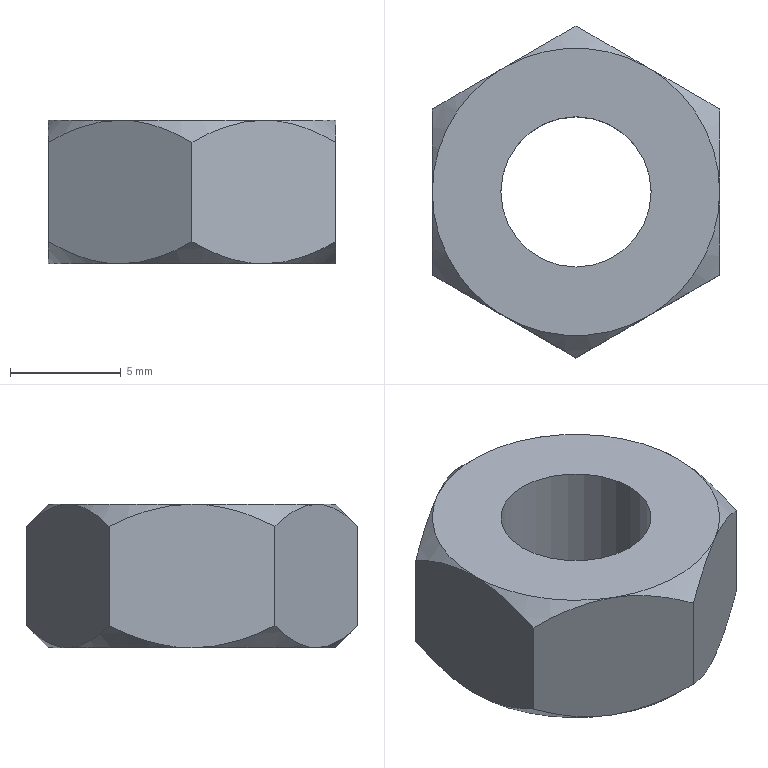Part | NX | 1 solid | 22 faces | box 13 x 15.011 x 6.5 mm | volume 707.016 mm3 | cone 12 | plane 8 | cylinder 2 | commonest cylinder face diameters 6.8 x2
STEP:
#1=CARTESIAN_POINT('',(3.25,-5.629,-3.25));
#2=VERTEX_POINT('',#1);
#3=CARTESIAN_POINT('',(6.5,0.,-3.25));
#4=VERTEX_POINT('',#3);
#5=CARTESIAN_POINT('',(0.,0.,-3.25));
#6=DIRECTION('',(0.,0.,1.));
#7=DIRECTION('',(0.5,-0.866,0.));
#8=AXIS2_PLACEMENT_3D('',#5,#6,#7);
#9=CIRCLE('',#8,6.5);
#10=EDGE_CURVE('',#2,#4,#9,.T.);
#11=ORIENTED_EDGE('',*,*,#10,.F.);
#12=CARTESIAN_POINT('',(-3.25,-5.629,-3.25));
#13=VERTEX_POINT('',#12);
#14=CARTESIAN_POINT('',(0.,0.,-3.25));
#15=DIRECTION('',(0.,0.,1.));
#16=DIRECTION('',(-0.5,-0.866,0.));
#17=AXIS2_PLACEMENT_3D('',#14,#15,#16);
#18=CIRCLE('',#17,6.5);
#19=EDGE_CURVE('',#13,#2,#18,.T.);
#20=ORIENTED_EDGE('',*,*,#19,.F.);
#21=CARTESIAN_POINT('',(-6.5,0.,-3.25));
#22=VERTEX_POINT('',#21);
#23=CARTESIAN_POINT('',(0.,0.,-3.25));
#24=DIRECTION('',(0.,0.,1.));
#25=DIRECTION('',(-1.,0.,0.));
#26=AXIS2_PLACEMENT_3D('',#23,#24,#25);
#27=CIRCLE('',#26,6.5);
#28=EDGE_CURVE('',#22,#13,#27,.T.);
#29=ORIENTED_EDGE('',*,*,#28,.F.);
#30=CARTESIAN_POINT('',(-3.25,5.629,-3.25));
#31=VERTEX_POINT('',#30);
#32=CARTESIAN_POINT('',(0.,0.,-3.25));
#33=DIRECTION('',(0.,0.,1.));
#34=DIRECTION('',(-0.5,0.866,0.));
#35=AXIS2_PLACEMENT_3D('',#32,#33,#34);
#36=CIRCLE('',#35,6.5);
#37=EDGE_CURVE('',#31,#22,#36,.T.);
#38=ORIENTED_EDGE('',*,*,#37,.F.);
#39=CARTESIAN_POINT('',(3.25,5.629,-3.25));
#40=VERTEX_POINT('',#39);
#41=CARTESIAN_POINT('',(0.,0.,-3.25));
#42=DIRECTION('',(0.,0.,1.));
#43=DIRECTION('',(0.5,0.866,0.));
#44=AXIS2_PLACEMENT_3D('',#41,#42,#43);
#45=CIRCLE('',#44,6.5);
#46=EDGE_CURVE('',#40,#31,#45,.T.);
#47=ORIENTED_EDGE('',*,*,#46,.F.);
#48=CARTESIAN_POINT('',(0.,0.,-3.25));
#49=DIRECTION('',(0.,0.,1.));
#50=DIRECTION('',(1.,0.,0.));
#51=AXIS2_PLACEMENT_3D('',#48,#49,#50);
#52=CIRCLE('',#51,6.5);
#53=EDGE_CURVE('',#4,#40,#52,.T.);
#54=ORIENTED_EDGE('',*,*,#53,.F.);
#55=EDGE_LOOP('',(#11,#20,#29,#38,#47,#54));
#56=FACE_BOUND('',#55,.T.);
#57=CARTESIAN_POINT('',(3.4,0.,-3.25));
#58=VERTEX_POINT('',#57);
#59=CARTESIAN_POINT('',(-3.4,0.,-3.25));
#60=VERTEX_POINT('',#59);
#61=CARTESIAN_POINT('',(0.,0.,-3.25));
#62=DIRECTION('',(0.,0.,-1.));
#63=DIRECTION('',(-1.,0.,0.));
#64=AXIS2_PLACEMENT_3D('',#61,#62,#63);
#65=CIRCLE('',#64,3.4);
#66=EDGE_CURVE('',#58,#60,#65,.T.);
#67=ORIENTED_EDGE('',*,*,#66,.F.);
#68=CARTESIAN_POINT('',(0.,0.,-3.25));
#69=DIRECTION('',(0.,0.,-1.));
#70=DIRECTION('',(-1.,0.,0.));
#71=AXIS2_PLACEMENT_3D('',#68,#69,#70);
#72=CIRCLE('',#71,3.4);
#73=EDGE_CURVE('',#60,#58,#72,.T.);
#74=ORIENTED_EDGE('',*,*,#73,.F.);
#75=EDGE_LOOP('',(#67,#74));
#76=FACE_BOUND('',#75,.T.);
#77=CARTESIAN_POINT('',(0.,0.,-3.25));
#78=DIRECTION('',(0.,0.,1.));
#79=DIRECTION('',(1.,0.,0.));
#80=AXIS2_PLACEMENT_3D('',#77,#78,#79);
#81=PLANE('',#80);
#82=ADVANCED_FACE('',(#56,#76),#81,.F.);
#83=CARTESIAN_POINT('',(6.5,-3.753,-2.244));
#84=VERTEX_POINT('',#83);
#85=CARTESIAN_POINT('',(3.25,-5.629,-3.25));
#86=CARTESIAN_POINT('',(3.764,-5.332,-3.25));
#87=CARTESIAN_POINT('',(4.854,-4.703,-3.071));
#88=CARTESIAN_POINT('',(5.912,-4.092,-2.584));
#89=CARTESIAN_POINT('',(6.5,-3.753,-2.244));
#90=B_SPLINE_CURVE_WITH_KNOTS('',3,(#85,#86,#87,#88,#89),.UNSPECIFIED.,.F.,.F.,(4,1,4),(0.,0.5,1.),.UNSPECIFIED.);
#91=EDGE_CURVE('',#2,#84,#90,.T.);
#92=ORIENTED_EDGE('',*,*,#91,.F.);
#93=ORIENTED_EDGE('',*,*,#10,.T.);
#94=CARTESIAN_POINT('',(6.5,-3.753,-2.244));
#95=CARTESIAN_POINT('',(6.5,-2.364,-2.939));
#96=CARTESIAN_POINT('',(6.5,-1.194,-3.25));
#97=CARTESIAN_POINT('',(6.5,0.,-3.25));
#98=B_SPLINE_CURVE_WITH_KNOTS('',3,(#94,#95,#96,#97),.UNSPECIFIED.,.F.,.F.,(4,4),(0.,1.),.UNSPECIFIED.);
#99=EDGE_CURVE('',#84,#4,#98,.T.);
#100=ORIENTED_EDGE('',*,*,#99,.F.);
#101=EDGE_LOOP('',(#92,#93,#100));
#102=FACE_BOUND('',#101,.T.);
#103=CARTESIAN_POINT('',(0.,0.,-2.747));
#104=DIRECTION('',(0.,0.,1.));
#105=DIRECTION('',(1.,0.,0.));
#106=AXIS2_PLACEMENT_3D('',#103,#104,#105);
#107=CONICAL_SURFACE('',#106,7.003,0.7854);
#108=ADVANCED_FACE('',(#102),#107,.T.);
#109=ORIENTED_EDGE('',*,*,#91,.T.);
#110=CARTESIAN_POINT('',(6.5,-3.753,2.244));
#111=VERTEX_POINT('',#110);
#112=CARTESIAN_POINT('',(6.5,-3.753,2.244));
#113=DIRECTION('',(0.,0.,-1.));
#114=VECTOR('',#113,1000.);
#115=LINE('',#112,#114);
#116=EDGE_CURVE('',#111,#84,#115,.T.);
#117=ORIENTED_EDGE('',*,*,#116,.F.);
#118=CARTESIAN_POINT('',(3.25,-5.629,3.25));
#119=VERTEX_POINT('',#118);
#120=CARTESIAN_POINT('',(6.5,-3.753,2.244));
#121=CARTESIAN_POINT('',(6.238,-3.904,2.396));
#122=CARTESIAN_POINT('',(5.711,-4.208,2.667));
#123=CARTESIAN_POINT('',(5.052,-4.589,2.946));
#124=CARTESIAN_POINT('',(4.099,-5.139,3.205));
#125=CARTESIAN_POINT('',(3.536,-5.464,3.25));
#126=CARTESIAN_POINT('',(3.25,-5.629,3.25));
#127=B_SPLINE_CURVE_WITH_KNOTS('',3,(#120,#121,#122,#123,#124,#125,#126),.UNSPECIFIED.,.F.,.F.,(4,1,1,1,4),(0.,0.25,0.5,0.75,1.),.UNSPECIFIED.);
#128=EDGE_CURVE('',#119,#111,#127,.F.);
#129=ORIENTED_EDGE('',*,*,#128,.F.);
#130=CARTESIAN_POINT('',(0.,-7.506,2.244));
#131=VERTEX_POINT('',#130);
#132=CARTESIAN_POINT('',(3.25,-5.629,3.25));
#133=CARTESIAN_POINT('',(2.736,-5.926,3.25));
#134=CARTESIAN_POINT('',(1.646,-6.555,3.071));
#135=CARTESIAN_POINT('',(0.5876,-7.166,2.584));
#136=CARTESIAN_POINT('',(0.,-7.506,2.244));
#137=B_SPLINE_CURVE_WITH_KNOTS('',3,(#132,#133,#134,#135,#136),.UNSPECIFIED.,.F.,.F.,(4,1,4),(0.,0.5,1.),.UNSPECIFIED.);
#138=EDGE_CURVE('',#119,#131,#137,.T.);
#139=ORIENTED_EDGE('',*,*,#138,.T.);
#140=CARTESIAN_POINT('',(0.,-7.506,-2.244));
#141=VERTEX_POINT('',#140);
#142=CARTESIAN_POINT('',(0.,-7.506,2.244));
#143=DIRECTION('',(0.,0.,-1.));
#144=VECTOR('',#143,1000.);
#145=LINE('',#142,#144);
#146=EDGE_CURVE('',#131,#141,#145,.T.);
#147=ORIENTED_EDGE('',*,*,#146,.T.);
#148=CARTESIAN_POINT('',(0.,-7.506,-2.244));
#149=CARTESIAN_POINT('',(0.1225,-7.435,-2.315));
#150=CARTESIAN_POINT('',(0.3631,-7.296,-2.448));
#151=CARTESIAN_POINT('',(0.7094,-7.096,-2.622));
#152=CARTESIAN_POINT('',(1.045,-6.902,-2.772));
#153=CARTESIAN_POINT('',(1.372,-6.714,-2.901));
#154=CARTESIAN_POINT('',(1.692,-6.529,-3.009));
#155=CARTESIAN_POINT('',(2.008,-6.346,-3.097));
#156=CARTESIAN_POINT('',(2.321,-6.165,-3.165));
#157=CARTESIAN_POINT('',(2.632,-5.986,-3.214));
#158=CARTESIAN_POINT('',(2.941,-5.807,-3.243));
#159=CARTESIAN_POINT('',(3.147,-5.689,-3.25));
#160=CARTESIAN_POINT('',(3.25,-5.629,-3.25));
#161=B_SPLINE_CURVE_WITH_KNOTS('',3,(#148,#149,#150,#151,#152,#153,#154,#155,#156,#157,#158,#159,#160),.UNSPECIFIED.,.F.,.F.,(4,1,1,1,1,1,1,1,1,1,4),(0.,0.1,0.2,0.3,0.4,0.5,0.6,0.7,0.8,0.9,1.),.UNSPECIFIED.);
#162=EDGE_CURVE('',#141,#2,#161,.T.);
#163=ORIENTED_EDGE('',*,*,#162,.T.);
#164=EDGE_LOOP('',(#109,#117,#129,#139,#147,#163));
#165=FACE_BOUND('',#164,.T.);
#166=CARTESIAN_POINT('',(0.,-7.506,-3.25));
#167=DIRECTION('',(0.5,-0.866,0.));
#168=DIRECTION('',(0.,0.,-1.));
#169=AXIS2_PLACEMENT_3D('',#166,#167,#168);
#170=PLANE('',#169);
#171=ADVANCED_FACE('',(#165),#170,.T.);
#172=CARTESIAN_POINT('',(-3.25,-5.629,-3.25));
#173=CARTESIAN_POINT('',(-2.736,-5.926,-3.25));
#174=CARTESIAN_POINT('',(-1.646,-6.555,-3.071));
#175=CARTESIAN_POINT('',(-0.5876,-7.166,-2.584));
#176=CARTESIAN_POINT('',(0.,-7.506,-2.244));
#177=B_SPLINE_CURVE_WITH_KNOTS('',3,(#172,#173,#174,#175,#176),.UNSPECIFIED.,.F.,.F.,(4,1,4),(0.,0.5,1.),.UNSPECIFIED.);
#178=EDGE_CURVE('',#13,#141,#177,.T.);
#179=ORIENTED_EDGE('',*,*,#178,.F.);
#180=ORIENTED_EDGE('',*,*,#19,.T.);
#181=ORIENTED_EDGE('',*,*,#162,.F.);
#182=EDGE_LOOP('',(#179,#180,#181));
#183=FACE_BOUND('',#182,.T.);
#184=CARTESIAN_POINT('',(0.,0.,-2.747));
#185=DIRECTION('',(0.,0.,1.));
#186=DIRECTION('',(1.,0.,0.));
#187=AXIS2_PLACEMENT_3D('',#184,#185,#186);
#188=CONICAL_SURFACE('',#187,7.003,0.7854);
#189=ADVANCED_FACE('',(#183),#188,.T.);
#190=ORIENTED_EDGE('',*,*,#178,.T.);
#191=ORIENTED_EDGE('',*,*,#146,.F.);
#192=CARTESIAN_POINT('',(-3.25,-5.629,3.25));
#193=VERTEX_POINT('',#192);
#194=CARTESIAN_POINT('',(0.,-7.506,2.244));
#195=CARTESIAN_POINT('',(-0.2618,-7.354,2.396));
#196=CARTESIAN_POINT('',(-0.7889,-7.05,2.667));
#197=CARTESIAN_POINT('',(-1.448,-6.669,2.946));
#198=CARTESIAN_POINT('',(-2.401,-6.119,3.205));
#199=CARTESIAN_POINT('',(-2.964,-5.794,3.25));
#200=CARTESIAN_POINT('',(-3.25,-5.629,3.25));
#201=B_SPLINE_CURVE_WITH_KNOTS('',3,(#194,#195,#196,#197,#198,#199,#200),.UNSPECIFIED.,.F.,.F.,(4,1,1,1,4),(0.,0.25,0.5,0.75,1.),.UNSPECIFIED.);
#202=EDGE_CURVE('',#193,#131,#201,.F.);
#203=ORIENTED_EDGE('',*,*,#202,.F.);
#204=CARTESIAN_POINT('',(-6.5,-3.753,2.244));
#205=VERTEX_POINT('',#204);
#206=CARTESIAN_POINT('',(-3.25,-5.629,3.25));
#207=CARTESIAN_POINT('',(-3.764,-5.332,3.25));
#208=CARTESIAN_POINT('',(-4.854,-4.703,3.071));
#209=CARTESIAN_POINT('',(-5.912,-4.092,2.584));
#210=CARTESIAN_POINT('',(-6.5,-3.753,2.244));
#211=B_SPLINE_CURVE_WITH_KNOTS('',3,(#206,#207,#208,#209,#210),.UNSPECIFIED.,.F.,.F.,(4,1,4),(0.,0.5,1.),.UNSPECIFIED.);
#212=EDGE_CURVE('',#193,#205,#211,.T.);
#213=ORIENTED_EDGE('',*,*,#212,.T.);
#214=CARTESIAN_POINT('',(-6.5,-3.753,-2.244));
#215=VERTEX_POINT('',#214);
#216=CARTESIAN_POINT('',(-6.5,-3.753,2.244));
#217=DIRECTION('',(0.,0.,-1.));
#218=VECTOR('',#217,1000.);
#219=LINE('',#216,#218);
#220=EDGE_CURVE('',#205,#215,#219,.T.);
#221=ORIENTED_EDGE('',*,*,#220,.T.);
#222=CARTESIAN_POINT('',(-6.5,-3.753,-2.244));
#223=CARTESIAN_POINT('',(-6.378,-3.823,-2.315));
#224=CARTESIAN_POINT('',(-6.137,-3.962,-2.448));
#225=CARTESIAN_POINT('',(-5.791,-4.162,-2.622));
#226=CARTESIAN_POINT('',(-5.455,-4.356,-2.772));
#227=CARTESIAN_POINT('',(-5.128,-4.545,-2.901));
#228=CARTESIAN_POINT('',(-4.808,-4.73,-3.009));
#229=CARTESIAN_POINT('',(-4.492,-4.912,-3.097));
#230=CARTESIAN_POINT('',(-4.179,-5.093,-3.165));
#231=CARTESIAN_POINT('',(-3.868,-5.272,-3.214));
#232=CARTESIAN_POINT('',(-3.559,-5.451,-3.243));
#233=CARTESIAN_POINT('',(-3.353,-5.57,-3.25));
#234=CARTESIAN_POINT('',(-3.25,-5.629,-3.25));
#235=B_SPLINE_CURVE_WITH_KNOTS('',3,(#222,#223,#224,#225,#226,#227,#228,#229,#230,#231,#232,#233,#234),.UNSPECIFIED.,.F.,.F.,(4,1,1,1,1,1,1,1,1,1,4),(0.,0.1,0.2,0.3,0.4,0.5,0.6,0.7,0.8,0.9,1.),.UNSPECIFIED.);
#236=EDGE_CURVE('',#215,#13,#235,.T.);
#237=ORIENTED_EDGE('',*,*,#236,.T.);
#238=EDGE_LOOP('',(#190,#191,#203,#213,#221,#237));
#239=FACE_BOUND('',#238,.T.);
#240=CARTESIAN_POINT('',(-6.5,-3.753,-3.25));
#241=DIRECTION('',(-0.5,-0.866,0.));
#242=DIRECTION('',(-0.866,0.5,0.));
#243=AXIS2_PLACEMENT_3D('',#240,#241,#242);
#244=PLANE('',#243);
#245=ADVANCED_FACE('',(#239),#244,.T.);
#246=CARTESIAN_POINT('',(-6.5,0.,-3.25));
#247=CARTESIAN_POINT('',(-6.5,-0.5936,-3.25));
#248=CARTESIAN_POINT('',(-6.5,-1.851,-3.071));
#249=CARTESIAN_POINT('',(-6.5,-3.074,-2.584));
#250=CARTESIAN_POINT('',(-6.5,-3.753,-2.244));
#251=B_SPLINE_CURVE_WITH_KNOTS('',3,(#246,#247,#248,#249,#250),.UNSPECIFIED.,.F.,.F.,(4,1,4),(0.,0.5,1.),.UNSPECIFIED.);
#252=EDGE_CURVE('',#22,#215,#251,.T.);
#253=ORIENTED_EDGE('',*,*,#252,.F.);
#254=ORIENTED_EDGE('',*,*,#28,.T.);
#255=ORIENTED_EDGE('',*,*,#236,.F.);
#256=EDGE_LOOP('',(#253,#254,#255));
#257=FACE_BOUND('',#256,.T.);
#258=CARTESIAN_POINT('',(0.,0.,-2.747));
#259=DIRECTION('',(0.,0.,1.));
#260=DIRECTION('',(1.,0.,0.));
#261=AXIS2_PLACEMENT_3D('',#258,#259,#260);
#262=CONICAL_SURFACE('',#261,7.003,0.7854);
#263=ADVANCED_FACE('',(#257),#262,.T.);
#264=ORIENTED_EDGE('',*,*,#252,.T.);
#265=ORIENTED_EDGE('',*,*,#220,.F.);
#266=CARTESIAN_POINT('',(-6.5,0.,3.25));
#267=VERTEX_POINT('',#266);
#268=CARTESIAN_POINT('',(-6.5,-3.753,2.244));
#269=CARTESIAN_POINT('',(-6.5,-3.447,2.397));
#270=CARTESIAN_POINT('',(-6.5,-2.834,2.671));
#271=CARTESIAN_POINT('',(-6.5,-2.057,2.953));
#272=CARTESIAN_POINT('',(-6.5,-0.9732,3.205));
#273=CARTESIAN_POINT('',(-6.5,-0.3273,3.25));
#274=CARTESIAN_POINT('',(-6.5,0.,3.25));
#275=B_SPLINE_CURVE_WITH_KNOTS('',3,(#268,#269,#270,#271,#272,#273,#274),.UNSPECIFIED.,.F.,.F.,(4,1,1,1,4),(0.,0.25,0.5,0.75,1.),.UNSPECIFIED.);
#276=EDGE_CURVE('',#267,#205,#275,.F.);
#277=ORIENTED_EDGE('',*,*,#276,.F.);
#278=CARTESIAN_POINT('',(-6.5,3.753,2.244));
#279=VERTEX_POINT('',#278);
#280=CARTESIAN_POINT('',(-6.5,0.,3.25));
#281=CARTESIAN_POINT('',(-6.5,0.5936,3.25));
#282=CARTESIAN_POINT('',(-6.5,1.851,3.071));
#283=CARTESIAN_POINT('',(-6.5,3.074,2.584));
#284=CARTESIAN_POINT('',(-6.5,3.753,2.244));
#285=B_SPLINE_CURVE_WITH_KNOTS('',3,(#280,#281,#282,#283,#284),.UNSPECIFIED.,.F.,.F.,(4,1,4),(0.,0.5,1.),.UNSPECIFIED.);
#286=EDGE_CURVE('',#267,#279,#285,.T.);
#287=ORIENTED_EDGE('',*,*,#286,.T.);
#288=CARTESIAN_POINT('',(-6.5,3.753,-2.244));
#289=VERTEX_POINT('',#288);
#290=CARTESIAN_POINT('',(-6.5,3.753,2.244));
#291=DIRECTION('',(0.,0.,-1.));
#292=VECTOR('',#291,1000.);
#293=LINE('',#290,#292);
#294=EDGE_CURVE('',#279,#289,#293,.T.);
#295=ORIENTED_EDGE('',*,*,#294,.T.);
#296=CARTESIAN_POINT('',(-6.5,3.753,-2.244));
#297=CARTESIAN_POINT('',(-6.5,2.364,-2.939));
#298=CARTESIAN_POINT('',(-6.5,1.194,-3.25));
#299=CARTESIAN_POINT('',(-6.5,0.,-3.25));
#300=B_SPLINE_CURVE_WITH_KNOTS('',3,(#296,#297,#298,#299),.UNSPECIFIED.,.F.,.F.,(4,4),(0.,1.),.UNSPECIFIED.);
#301=EDGE_CURVE('',#289,#22,#300,.T.);
#302=ORIENTED_EDGE('',*,*,#301,.T.);
#303=EDGE_LOOP('',(#264,#265,#277,#287,#295,#302));
#304=FACE_BOUND('',#303,.T.);
#305=CARTESIAN_POINT('',(-6.5,3.753,-3.25));
#306=DIRECTION('',(-1.,0.,0.));
#307=DIRECTION('',(0.,0.,1.));
#308=AXIS2_PLACEMENT_3D('',#305,#306,#307);
#309=PLANE('',#308);
#310=ADVANCED_FACE('',(#304),#309,.T.);
#311=CARTESIAN_POINT('',(-3.25,5.629,-3.25));
#312=CARTESIAN_POINT('',(-3.764,5.332,-3.25));
#313=CARTESIAN_POINT('',(-4.854,4.703,-3.071));
#314=CARTESIAN_POINT('',(-5.912,4.092,-2.584));
#315=CARTESIAN_POINT('',(-6.5,3.753,-2.244));
#316=B_SPLINE_CURVE_WITH_KNOTS('',3,(#311,#312,#313,#314,#315),.UNSPECIFIED.,.F.,.F.,(4,1,4),(0.,0.5,1.),.UNSPECIFIED.);
#317=EDGE_CURVE('',#31,#289,#316,.T.);
#318=ORIENTED_EDGE('',*,*,#317,.F.);
#319=ORIENTED_EDGE('',*,*,#37,.T.);
#320=ORIENTED_EDGE('',*,*,#301,.F.);
#321=EDGE_LOOP('',(#318,#319,#320));
#322=FACE_BOUND('',#321,.T.);
#323=CARTESIAN_POINT('',(0.,0.,-2.747));
#324=DIRECTION('',(0.,0.,1.));
#325=DIRECTION('',(1.,0.,0.));
#326=AXIS2_PLACEMENT_3D('',#323,#324,#325);
#327=CONICAL_SURFACE('',#326,7.003,0.7854);
#328=ADVANCED_FACE('',(#322),#327,.T.);
#329=ORIENTED_EDGE('',*,*,#317,.T.);
#330=ORIENTED_EDGE('',*,*,#294,.F.);
#331=CARTESIAN_POINT('',(-3.25,5.629,3.25));
#332=VERTEX_POINT('',#331);
#333=CARTESIAN_POINT('',(-6.5,3.753,2.244));
#334=CARTESIAN_POINT('',(-6.238,3.904,2.396));
#335=CARTESIAN_POINT('',(-5.711,4.208,2.667));
#336=CARTESIAN_POINT('',(-5.052,4.589,2.946));
#337=CARTESIAN_POINT('',(-4.099,5.139,3.205));
#338=CARTESIAN_POINT('',(-3.536,5.464,3.25));
#339=CARTESIAN_POINT('',(-3.25,5.629,3.25));
#340=B_SPLINE_CURVE_WITH_KNOTS('',3,(#333,#334,#335,#336,#337,#338,#339),.UNSPECIFIED.,.F.,.F.,(4,1,1,1,4),(0.,0.25,0.5,0.75,1.),.UNSPECIFIED.);
#341=EDGE_CURVE('',#332,#279,#340,.F.);
#342=ORIENTED_EDGE('',*,*,#341,.F.);
#343=CARTESIAN_POINT('',(0.,7.506,2.244));
#344=VERTEX_POINT('',#343);
#345=CARTESIAN_POINT('',(-3.25,5.629,3.25));
#346=CARTESIAN_POINT('',(-2.736,5.926,3.25));
#347=CARTESIAN_POINT('',(-1.646,6.555,3.071));
#348=CARTESIAN_POINT('',(-0.5876,7.166,2.584));
#349=CARTESIAN_POINT('',(0.,7.506,2.244));
#350=B_SPLINE_CURVE_WITH_KNOTS('',3,(#345,#346,#347,#348,#349),.UNSPECIFIED.,.F.,.F.,(4,1,4),(0.,0.5,1.),.UNSPECIFIED.);
#351=EDGE_CURVE('',#332,#344,#350,.T.);
#352=ORIENTED_EDGE('',*,*,#351,.T.);
#353=CARTESIAN_POINT('',(0.,7.506,-2.244));
#354=VERTEX_POINT('',#353);
#355=CARTESIAN_POINT('',(0.,7.506,2.244));
#356=DIRECTION('',(0.,0.,-1.));
#357=VECTOR('',#356,1000.);
#358=LINE('',#355,#357);
#359=EDGE_CURVE('',#344,#354,#358,.T.);
#360=ORIENTED_EDGE('',*,*,#359,.T.);
#361=CARTESIAN_POINT('',(0.,7.506,-2.244));
#362=CARTESIAN_POINT('',(-0.1225,7.435,-2.315));
#363=CARTESIAN_POINT('',(-0.3631,7.296,-2.448));
#364=CARTESIAN_POINT('',(-0.7094,7.096,-2.622));
#365=CARTESIAN_POINT('',(-1.045,6.902,-2.772));
#366=CARTESIAN_POINT('',(-1.372,6.714,-2.901));
#367=CARTESIAN_POINT('',(-1.692,6.529,-3.009));
#368=CARTESIAN_POINT('',(-2.008,6.346,-3.097));
#369=CARTESIAN_POINT('',(-2.321,6.165,-3.165));
#370=CARTESIAN_POINT('',(-2.632,5.986,-3.214));
#371=CARTESIAN_POINT('',(-2.941,5.807,-3.243));
#372=CARTESIAN_POINT('',(-3.147,5.689,-3.25));
#373=CARTESIAN_POINT('',(-3.25,5.629,-3.25));
#374=B_SPLINE_CURVE_WITH_KNOTS('',3,(#361,#362,#363,#364,#365,#366,#367,#368,#369,#370,#371,#372,#373),.UNSPECIFIED.,.F.,.F.,(4,1,1,1,1,1,1,1,1,1,4),(0.,0.1,0.2,0.3,0.4,0.5,0.6,0.7,0.8,0.9,1.),.UNSPECIFIED.);
#375=EDGE_CURVE('',#354,#31,#374,.T.);
#376=ORIENTED_EDGE('',*,*,#375,.T.);
#377=EDGE_LOOP('',(#329,#330,#342,#352,#360,#376));
#378=FACE_BOUND('',#377,.T.);
#379=CARTESIAN_POINT('',(0.,7.506,-3.25));
#380=DIRECTION('',(-0.5,0.866,0.));
#381=DIRECTION('',(0.,0.,1.));
#382=AXIS2_PLACEMENT_3D('',#379,#380,#381);
#383=PLANE('',#382);
#384=ADVANCED_FACE('',(#378),#383,.T.);
#385=CARTESIAN_POINT('',(3.25,5.629,-3.25));
#386=CARTESIAN_POINT('',(2.736,5.926,-3.25));
#387=CARTESIAN_POINT('',(1.646,6.555,-3.071));
#388=CARTESIAN_POINT('',(0.5876,7.166,-2.584));
#389=CARTESIAN_POINT('',(0.,7.506,-2.244));
#390=B_SPLINE_CURVE_WITH_KNOTS('',3,(#385,#386,#387,#388,#389),.UNSPECIFIED.,.F.,.F.,(4,1,4),(0.,0.5,1.),.UNSPECIFIED.);
#391=EDGE_CURVE('',#40,#354,#390,.T.);
#392=ORIENTED_EDGE('',*,*,#391,.F.);
#393=ORIENTED_EDGE('',*,*,#46,.T.);
#394=ORIENTED_EDGE('',*,*,#375,.F.);
#395=EDGE_LOOP('',(#392,#393,#394));
#396=FACE_BOUND('',#395,.T.);
#397=CARTESIAN_POINT('',(0.,0.,-2.747));
#398=DIRECTION('',(0.,0.,1.));
#399=DIRECTION('',(1.,0.,0.));
#400=AXIS2_PLACEMENT_3D('',#397,#398,#399);
#401=CONICAL_SURFACE('',#400,7.003,0.7854);
#402=ADVANCED_FACE('',(#396),#401,.T.);
#403=ORIENTED_EDGE('',*,*,#391,.T.);
#404=ORIENTED_EDGE('',*,*,#359,.F.);
#405=CARTESIAN_POINT('',(3.25,5.629,3.25));
#406=VERTEX_POINT('',#405);
#407=CARTESIAN_POINT('',(0.,7.506,2.244));
#408=CARTESIAN_POINT('',(0.2618,7.354,2.396));
#409=CARTESIAN_POINT('',(0.7889,7.05,2.667));
#410=CARTESIAN_POINT('',(1.448,6.669,2.946));
#411=CARTESIAN_POINT('',(2.401,6.119,3.205));
#412=CARTESIAN_POINT('',(2.964,5.794,3.25));
#413=CARTESIAN_POINT('',(3.25,5.629,3.25));
#414=B_SPLINE_CURVE_WITH_KNOTS('',3,(#407,#408,#409,#410,#411,#412,#413),.UNSPECIFIED.,.F.,.F.,(4,1,1,1,4),(0.,0.25,0.5,0.75,1.),.UNSPECIFIED.);
#415=EDGE_CURVE('',#406,#344,#414,.F.);
#416=ORIENTED_EDGE('',*,*,#415,.F.);
#417=CARTESIAN_POINT('',(6.5,3.753,2.244));
#418=VERTEX_POINT('',#417);
#419=CARTESIAN_POINT('',(3.25,5.629,3.25));
#420=CARTESIAN_POINT('',(3.764,5.332,3.25));
#421=CARTESIAN_POINT('',(4.854,4.703,3.071));
#422=CARTESIAN_POINT('',(5.912,4.092,2.584));
#423=CARTESIAN_POINT('',(6.5,3.753,2.244));
#424=B_SPLINE_CURVE_WITH_KNOTS('',3,(#419,#420,#421,#422,#423),.UNSPECIFIED.,.F.,.F.,(4,1,4),(0.,0.5,1.),.UNSPECIFIED.);
#425=EDGE_CURVE('',#406,#418,#424,.T.);
#426=ORIENTED_EDGE('',*,*,#425,.T.);
#427=CARTESIAN_POINT('',(6.5,3.753,-2.244));
#428=VERTEX_POINT('',#427);
#429=CARTESIAN_POINT('',(6.5,3.753,2.244));
#430=DIRECTION('',(0.,0.,-1.));
#431=VECTOR('',#430,1000.);
#432=LINE('',#429,#431);
#433=EDGE_CURVE('',#418,#428,#432,.T.);
#434=ORIENTED_EDGE('',*,*,#433,.T.);
#435=CARTESIAN_POINT('',(6.5,3.753,-2.244));
#436=CARTESIAN_POINT('',(6.378,3.823,-2.315));
#437=CARTESIAN_POINT('',(6.137,3.962,-2.448));
#438=CARTESIAN_POINT('',(5.791,4.162,-2.622));
#439=CARTESIAN_POINT('',(5.455,4.356,-2.772));
#440=CARTESIAN_POINT('',(5.128,4.545,-2.901));
#441=CARTESIAN_POINT('',(4.808,4.73,-3.009));
#442=CARTESIAN_POINT('',(4.492,4.912,-3.097));
#443=CARTESIAN_POINT('',(4.179,5.093,-3.165));
#444=CARTESIAN_POINT('',(3.868,5.272,-3.214));
#445=CARTESIAN_POINT('',(3.559,5.451,-3.243));
#446=CARTESIAN_POINT('',(3.353,5.57,-3.25));
#447=CARTESIAN_POINT('',(3.25,5.629,-3.25));
#448=B_SPLINE_CURVE_WITH_KNOTS('',3,(#435,#436,#437,#438,#439,#440,#441,#442,#443,#444,#445,#446,#447),.UNSPECIFIED.,.F.,.F.,(4,1,1,1,1,1,1,1,1,1,4),(0.,0.1,0.2,0.3,0.4,0.5,0.6,0.7,0.8,0.9,1.),.UNSPECIFIED.);
#449=EDGE_CURVE('',#428,#40,#448,.T.);
#450=ORIENTED_EDGE('',*,*,#449,.T.);
#451=EDGE_LOOP('',(#403,#404,#416,#426,#434,#450));
#452=FACE_BOUND('',#451,.T.);
#453=CARTESIAN_POINT('',(6.5,3.753,-3.25));
#454=DIRECTION('',(0.5,0.866,0.));
#455=DIRECTION('',(0.,0.,-1.));
#456=AXIS2_PLACEMENT_3D('',#453,#454,#455);
#457=PLANE('',#456);
#458=ADVANCED_FACE('',(#452),#457,.T.);
#459=CARTESIAN_POINT('',(6.5,0.,-3.25));
#460=CARTESIAN_POINT('',(6.5,0.5936,-3.25));
#461=CARTESIAN_POINT('',(6.5,1.851,-3.071));
#462=CARTESIAN_POINT('',(6.5,3.074,-2.584));
#463=CARTESIAN_POINT('',(6.5,3.753,-2.244));
#464=B_SPLINE_CURVE_WITH_KNOTS('',3,(#459,#460,#461,#462,#463),.UNSPECIFIED.,.F.,.F.,(4,1,4),(0.,0.5,1.),.UNSPECIFIED.);
#465=EDGE_CURVE('',#4,#428,#464,.T.);
#466=ORIENTED_EDGE('',*,*,#465,.F.);
#467=ORIENTED_EDGE('',*,*,#53,.T.);
#468=ORIENTED_EDGE('',*,*,#449,.F.);
#469=EDGE_LOOP('',(#466,#467,#468));
#470=FACE_BOUND('',#469,.T.);
#471=CARTESIAN_POINT('',(0.,0.,-2.747));
#472=DIRECTION('',(0.,0.,1.));
#473=DIRECTION('',(1.,0.,0.));
#474=AXIS2_PLACEMENT_3D('',#471,#472,#473);
#475=CONICAL_SURFACE('',#474,7.003,0.7854);
#476=ADVANCED_FACE('',(#470),#475,.T.);
#477=ORIENTED_EDGE('',*,*,#99,.T.);
#478=ORIENTED_EDGE('',*,*,#465,.T.);
#479=ORIENTED_EDGE('',*,*,#433,.F.);
#480=CARTESIAN_POINT('',(6.5,0.,3.25));
#481=VERTEX_POINT('',#480);
#482=CARTESIAN_POINT('',(6.5,3.753,2.244));
#483=CARTESIAN_POINT('',(6.5,3.447,2.397));
#484=CARTESIAN_POINT('',(6.5,2.834,2.671));
#485=CARTESIAN_POINT('',(6.5,2.057,2.953));
#486=CARTESIAN_POINT('',(6.5,0.9732,3.205));
#487=CARTESIAN_POINT('',(6.5,0.3273,3.25));
#488=CARTESIAN_POINT('',(6.5,0.,3.25));
#489=B_SPLINE_CURVE_WITH_KNOTS('',3,(#482,#483,#484,#485,#486,#487,#488),.UNSPECIFIED.,.F.,.F.,(4,1,1,1,4),(0.,0.25,0.5,0.75,1.),.UNSPECIFIED.);
#490=EDGE_CURVE('',#481,#418,#489,.F.);
#491=ORIENTED_EDGE('',*,*,#490,.F.);
#492=CARTESIAN_POINT('',(6.5,0.,3.25));
#493=CARTESIAN_POINT('',(6.5,-0.5936,3.25));
#494=CARTESIAN_POINT('',(6.5,-1.851,3.071));
#495=CARTESIAN_POINT('',(6.5,-3.074,2.584));
#496=CARTESIAN_POINT('',(6.5,-3.753,2.244));
#497=B_SPLINE_CURVE_WITH_KNOTS('',3,(#492,#493,#494,#495,#496),.UNSPECIFIED.,.F.,.F.,(4,1,4),(0.,0.5,1.),.UNSPECIFIED.);
#498=EDGE_CURVE('',#481,#111,#497,.T.);
#499=ORIENTED_EDGE('',*,*,#498,.T.);
#500=ORIENTED_EDGE('',*,*,#116,.T.);
#501=EDGE_LOOP('',(#477,#478,#479,#491,#499,#500));
#502=FACE_BOUND('',#501,.T.);
#503=CARTESIAN_POINT('',(6.5,-3.753,-3.25));
#504=DIRECTION('',(1.,0.,0.));
#505=DIRECTION('',(0.,1.,0.));
#506=AXIS2_PLACEMENT_3D('',#503,#504,#505);
#507=PLANE('',#506);
#508=ADVANCED_FACE('',(#502),#507,.T.);
#509=ORIENTED_EDGE('',*,*,#498,.F.);
#510=CARTESIAN_POINT('',(0.,0.,3.25));
#511=DIRECTION('',(0.,0.,-1.));
#512=DIRECTION('',(1.,0.,0.));
#513=AXIS2_PLACEMENT_3D('',#510,#511,#512);
#514=CIRCLE('',#513,6.5);
#515=EDGE_CURVE('',#481,#119,#514,.T.);
#516=ORIENTED_EDGE('',*,*,#515,.T.);
#517=ORIENTED_EDGE('',*,*,#128,.T.);
#518=EDGE_LOOP('',(#509,#516,#517));
#519=FACE_BOUND('',#518,.T.);
#520=CARTESIAN_POINT('',(0.,0.,2.747));
#521=DIRECTION('',(0.,0.,-1.));
#522=DIRECTION('',(-1.,0.,0.));
#523=AXIS2_PLACEMENT_3D('',#520,#521,#522);
#524=CONICAL_SURFACE('',#523,7.003,0.7854);
#525=ADVANCED_FACE('',(#519),#524,.T.);
#526=ORIENTED_EDGE('',*,*,#515,.F.);
#527=CARTESIAN_POINT('',(0.,0.,3.25));
#528=DIRECTION('',(0.,0.,-1.));
#529=DIRECTION('',(0.5,0.866,0.));
#530=AXIS2_PLACEMENT_3D('',#527,#528,#529);
#531=CIRCLE('',#530,6.5);
#532=EDGE_CURVE('',#406,#481,#531,.T.);
#533=ORIENTED_EDGE('',*,*,#532,.F.);
#534=CARTESIAN_POINT('',(0.,0.,3.25));
#535=DIRECTION('',(0.,0.,-1.));
#536=DIRECTION('',(-0.5,0.866,0.));
#537=AXIS2_PLACEMENT_3D('',#534,#535,#536);
#538=CIRCLE('',#537,6.5);
#539=EDGE_CURVE('',#332,#406,#538,.T.);
#540=ORIENTED_EDGE('',*,*,#539,.F.);
#541=CARTESIAN_POINT('',(0.,0.,3.25));
#542=DIRECTION('',(0.,0.,-1.));
#543=DIRECTION('',(-1.,0.,0.));
#544=AXIS2_PLACEMENT_3D('',#541,#542,#543);
#545=CIRCLE('',#544,6.5);
#546=EDGE_CURVE('',#267,#332,#545,.T.);
#547=ORIENTED_EDGE('',*,*,#546,.F.);
#548=CARTESIAN_POINT('',(0.,0.,3.25));
#549=DIRECTION('',(0.,0.,-1.));
#550=DIRECTION('',(-0.5,-0.866,0.));
#551=AXIS2_PLACEMENT_3D('',#548,#549,#550);
#552=CIRCLE('',#551,6.5);
#553=EDGE_CURVE('',#193,#267,#552,.T.);
#554=ORIENTED_EDGE('',*,*,#553,.F.);
#555=CARTESIAN_POINT('',(0.,0.,3.25));
#556=DIRECTION('',(0.,0.,-1.));
#557=DIRECTION('',(0.5,-0.866,0.));
#558=AXIS2_PLACEMENT_3D('',#555,#556,#557);
#559=CIRCLE('',#558,6.5);
#560=EDGE_CURVE('',#119,#193,#559,.T.);
#561=ORIENTED_EDGE('',*,*,#560,.F.);
#562=EDGE_LOOP('',(#526,#533,#540,#547,#554,#561));
#563=FACE_BOUND('',#562,.T.);
#564=CARTESIAN_POINT('',(3.4,0.,3.25));
#565=VERTEX_POINT('',#564);
#566=CARTESIAN_POINT('',(-3.4,0.,3.25));
#567=VERTEX_POINT('',#566);
#568=CARTESIAN_POINT('',(0.,0.,3.25));
#569=DIRECTION('',(0.,0.,1.));
#570=DIRECTION('',(1.,0.,0.));
#571=AXIS2_PLACEMENT_3D('',#568,#569,#570);
#572=CIRCLE('',#571,3.4);
#573=EDGE_CURVE('',#565,#567,#572,.T.);
#574=ORIENTED_EDGE('',*,*,#573,.F.);
#575=CARTESIAN_POINT('',(0.,0.,3.25));
#576=DIRECTION('',(0.,0.,1.));
#577=DIRECTION('',(1.,0.,0.));
#578=AXIS2_PLACEMENT_3D('',#575,#576,#577);
#579=CIRCLE('',#578,3.4);
#580=EDGE_CURVE('',#567,#565,#579,.T.);
#581=ORIENTED_EDGE('',*,*,#580,.F.);
#582=EDGE_LOOP('',(#574,#581));
#583=FACE_BOUND('',#582,.T.);
#584=CARTESIAN_POINT('',(0.,0.,3.25));
#585=DIRECTION('',(0.,0.,1.));
#586=DIRECTION('',(1.,0.,0.));
#587=AXIS2_PLACEMENT_3D('',#584,#585,#586);
#588=PLANE('',#587);
#589=ADVANCED_FACE('',(#563,#583),#588,.T.);
#590=ORIENTED_EDGE('',*,*,#138,.F.);
#591=ORIENTED_EDGE('',*,*,#560,.T.);
#592=ORIENTED_EDGE('',*,*,#202,.T.);
#593=EDGE_LOOP('',(#590,#591,#592));
#594=FACE_BOUND('',#593,.T.);
#595=CARTESIAN_POINT('',(0.,0.,2.747));
#596=DIRECTION('',(0.,0.,-1.));
#597=DIRECTION('',(-1.,0.,0.));
#598=AXIS2_PLACEMENT_3D('',#595,#596,#597);
#599=CONICAL_SURFACE('',#598,7.003,0.7854);
#600=ADVANCED_FACE('',(#594),#599,.T.);
#601=ORIENTED_EDGE('',*,*,#212,.F.);
#602=ORIENTED_EDGE('',*,*,#553,.T.);
#603=ORIENTED_EDGE('',*,*,#276,.T.);
#604=EDGE_LOOP('',(#601,#602,#603));
#605=FACE_BOUND('',#604,.T.);
#606=CARTESIAN_POINT('',(0.,0.,2.747));
#607=DIRECTION('',(0.,0.,-1.));
#608=DIRECTION('',(-1.,0.,0.));
#609=AXIS2_PLACEMENT_3D('',#606,#607,#608);
#610=CONICAL_SURFACE('',#609,7.003,0.7854);
#611=ADVANCED_FACE('',(#605),#610,.T.);
#612=ORIENTED_EDGE('',*,*,#286,.F.);
#613=ORIENTED_EDGE('',*,*,#546,.T.);
#614=ORIENTED_EDGE('',*,*,#341,.T.);
#615=EDGE_LOOP('',(#612,#613,#614));
#616=FACE_BOUND('',#615,.T.);
#617=CARTESIAN_POINT('',(0.,0.,2.747));
#618=DIRECTION('',(0.,0.,-1.));
#619=DIRECTION('',(-1.,0.,0.));
#620=AXIS2_PLACEMENT_3D('',#617,#618,#619);
#621=CONICAL_SURFACE('',#620,7.003,0.7854);
#622=ADVANCED_FACE('',(#616),#621,.T.);
#623=ORIENTED_EDGE('',*,*,#351,.F.);
#624=ORIENTED_EDGE('',*,*,#539,.T.);
#625=ORIENTED_EDGE('',*,*,#415,.T.);
#626=EDGE_LOOP('',(#623,#624,#625));
#627=FACE_BOUND('',#626,.T.);
#628=CARTESIAN_POINT('',(0.,0.,2.747));
#629=DIRECTION('',(0.,0.,-1.));
#630=DIRECTION('',(-1.,0.,0.));
#631=AXIS2_PLACEMENT_3D('',#628,#629,#630);
#632=CONICAL_SURFACE('',#631,7.003,0.7854);
#633=ADVANCED_FACE('',(#627),#632,.T.);
#634=ORIENTED_EDGE('',*,*,#425,.F.);
#635=ORIENTED_EDGE('',*,*,#532,.T.);
#636=ORIENTED_EDGE('',*,*,#490,.T.);
#637=EDGE_LOOP('',(#634,#635,#636));
#638=FACE_BOUND('',#637,.T.);
#639=CARTESIAN_POINT('',(0.,0.,2.747));
#640=DIRECTION('',(0.,0.,-1.));
#641=DIRECTION('',(-1.,0.,0.));
#642=AXIS2_PLACEMENT_3D('',#639,#640,#641);
#643=CONICAL_SURFACE('',#642,7.003,0.7854);
#644=ADVANCED_FACE('',(#638),#643,.T.);
#645=ORIENTED_EDGE('',*,*,#66,.T.);
#646=CARTESIAN_POINT('',(-3.4,0.,-4.258));
#647=DIRECTION('',(0.,0.,1.));
#648=VECTOR('',#647,1000.);
#649=LINE('',#646,#648);
#650=EDGE_CURVE('',#567,#60,#649,.F.);
#651=ORIENTED_EDGE('',*,*,#650,.F.);
#652=ORIENTED_EDGE('',*,*,#580,.T.);
#653=CARTESIAN_POINT('',(3.4,0.,-4.258));
#654=DIRECTION('',(0.,0.,1.));
#655=VECTOR('',#654,1000.);
#656=LINE('',#653,#655);
#657=EDGE_CURVE('',#565,#58,#656,.F.);
#658=ORIENTED_EDGE('',*,*,#657,.T.);
#659=EDGE_LOOP('',(#645,#651,#652,#658));
#660=FACE_BOUND('',#659,.T.);
#661=CARTESIAN_POINT('',(0.,0.,-4.258));
#662=DIRECTION('',(0.,0.,1.));
#663=DIRECTION('',(-1.,0.,0.));
#664=AXIS2_PLACEMENT_3D('',#661,#662,#663);
#665=CYLINDRICAL_SURFACE('',#664,3.4);
#666=ADVANCED_FACE('',(#660),#665,.F.);
#667=ORIENTED_EDGE('',*,*,#573,.T.);
#668=ORIENTED_EDGE('',*,*,#650,.T.);
#669=ORIENTED_EDGE('',*,*,#73,.T.);
#670=ORIENTED_EDGE('',*,*,#657,.F.);
#671=EDGE_LOOP('',(#667,#668,#669,#670));
#672=FACE_BOUND('',#671,.T.);
#673=CARTESIAN_POINT('',(0.,0.,-4.258));
#674=DIRECTION('',(0.,0.,1.));
#675=DIRECTION('',(-1.,0.,0.));
#676=AXIS2_PLACEMENT_3D('',#673,#674,#675);
#677=CYLINDRICAL_SURFACE('',#676,3.4);
#678=ADVANCED_FACE('',(#672),#677,.F.);
#679=CLOSED_SHELL('',(#82,#108,#171,#189,#245,#263,#310,#328,#384,#402,#458,#476,#508,#525,#589,#600,#611,#622,#633,#644,#666,#678));
#680=MANIFOLD_SOLID_BREP('',#679);
#681=(LENGTH_UNIT()NAMED_UNIT(*)SI_UNIT(.MILLI.,.METRE.));
#682=UNCERTAINTY_MEASURE_WITH_UNIT(LENGTH_MEASURE(0.0508),#681,'','');
#683=(NAMED_UNIT(*)PLANE_ANGLE_UNIT()SI_UNIT($,.RADIAN.));
#684=(NAMED_UNIT(*)SI_UNIT($,.STERADIAN.)SOLID_ANGLE_UNIT());
#685=(GEOMETRIC_REPRESENTATION_CONTEXT(3)GLOBAL_UNCERTAINTY_ASSIGNED_CONTEXT((#682))GLOBAL_UNIT_ASSIGNED_CONTEXT((#681,#683,#684))REPRESENTATION_CONTEXT('',''));
#686=ADVANCED_BREP_SHAPE_REPRESENTATION('',(#680),#685);